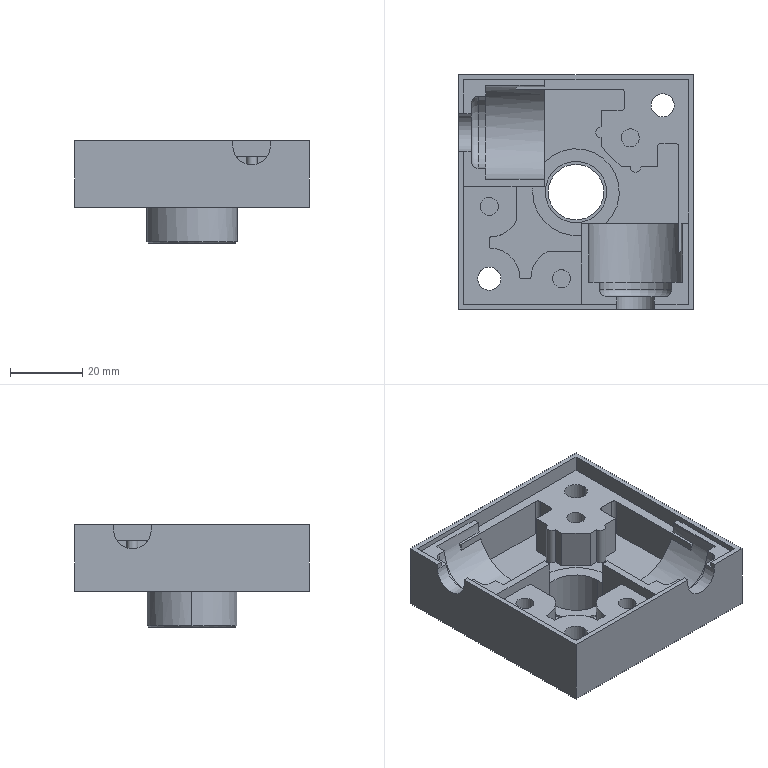Part | STEP file | Gear Box.1(Lower).stp | 1 solid | 96 faces | box 65 x 65 x 28.5 mm | volume 40735 mm3 | plane 58 | cylinder 34 | cone 2 | torus 2 | commonest cylinder face diameters 5 x6 17 x5 2 x4 6.4 x4 24 x3 3 x2